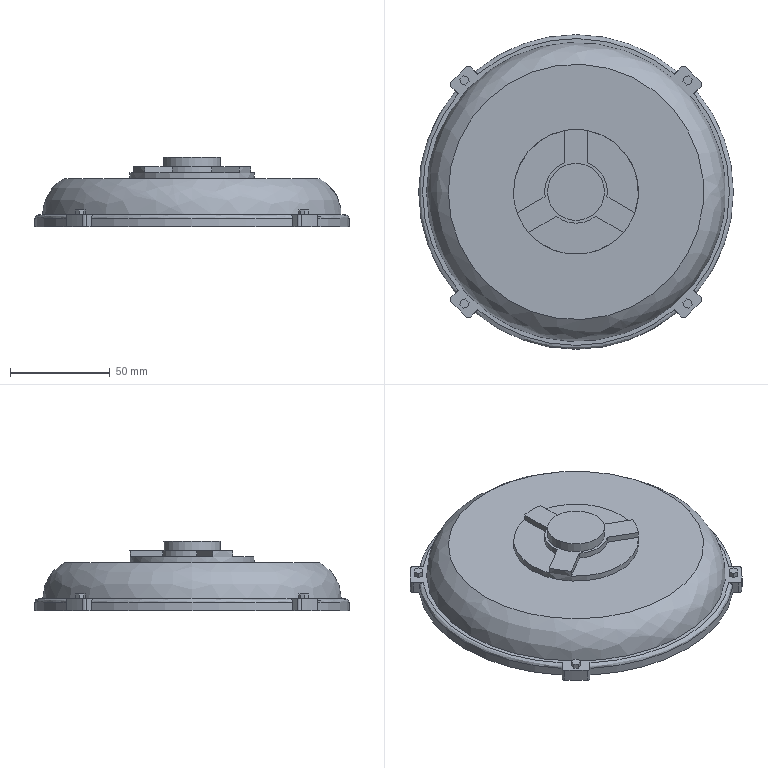Part | STEP file | Y2_B3_FL_80_1.step 4 | 1 solid | 76 faces | box 157.5 x 157.5 x 35 mm | volume 429524 mm3 | plane 50 | cylinder 21 | spline 5 | commonest cylinder face diameters 2.8 x8 157.5 x4 166.25 x4 31.35 x3 28.5 x1 62.542 x1